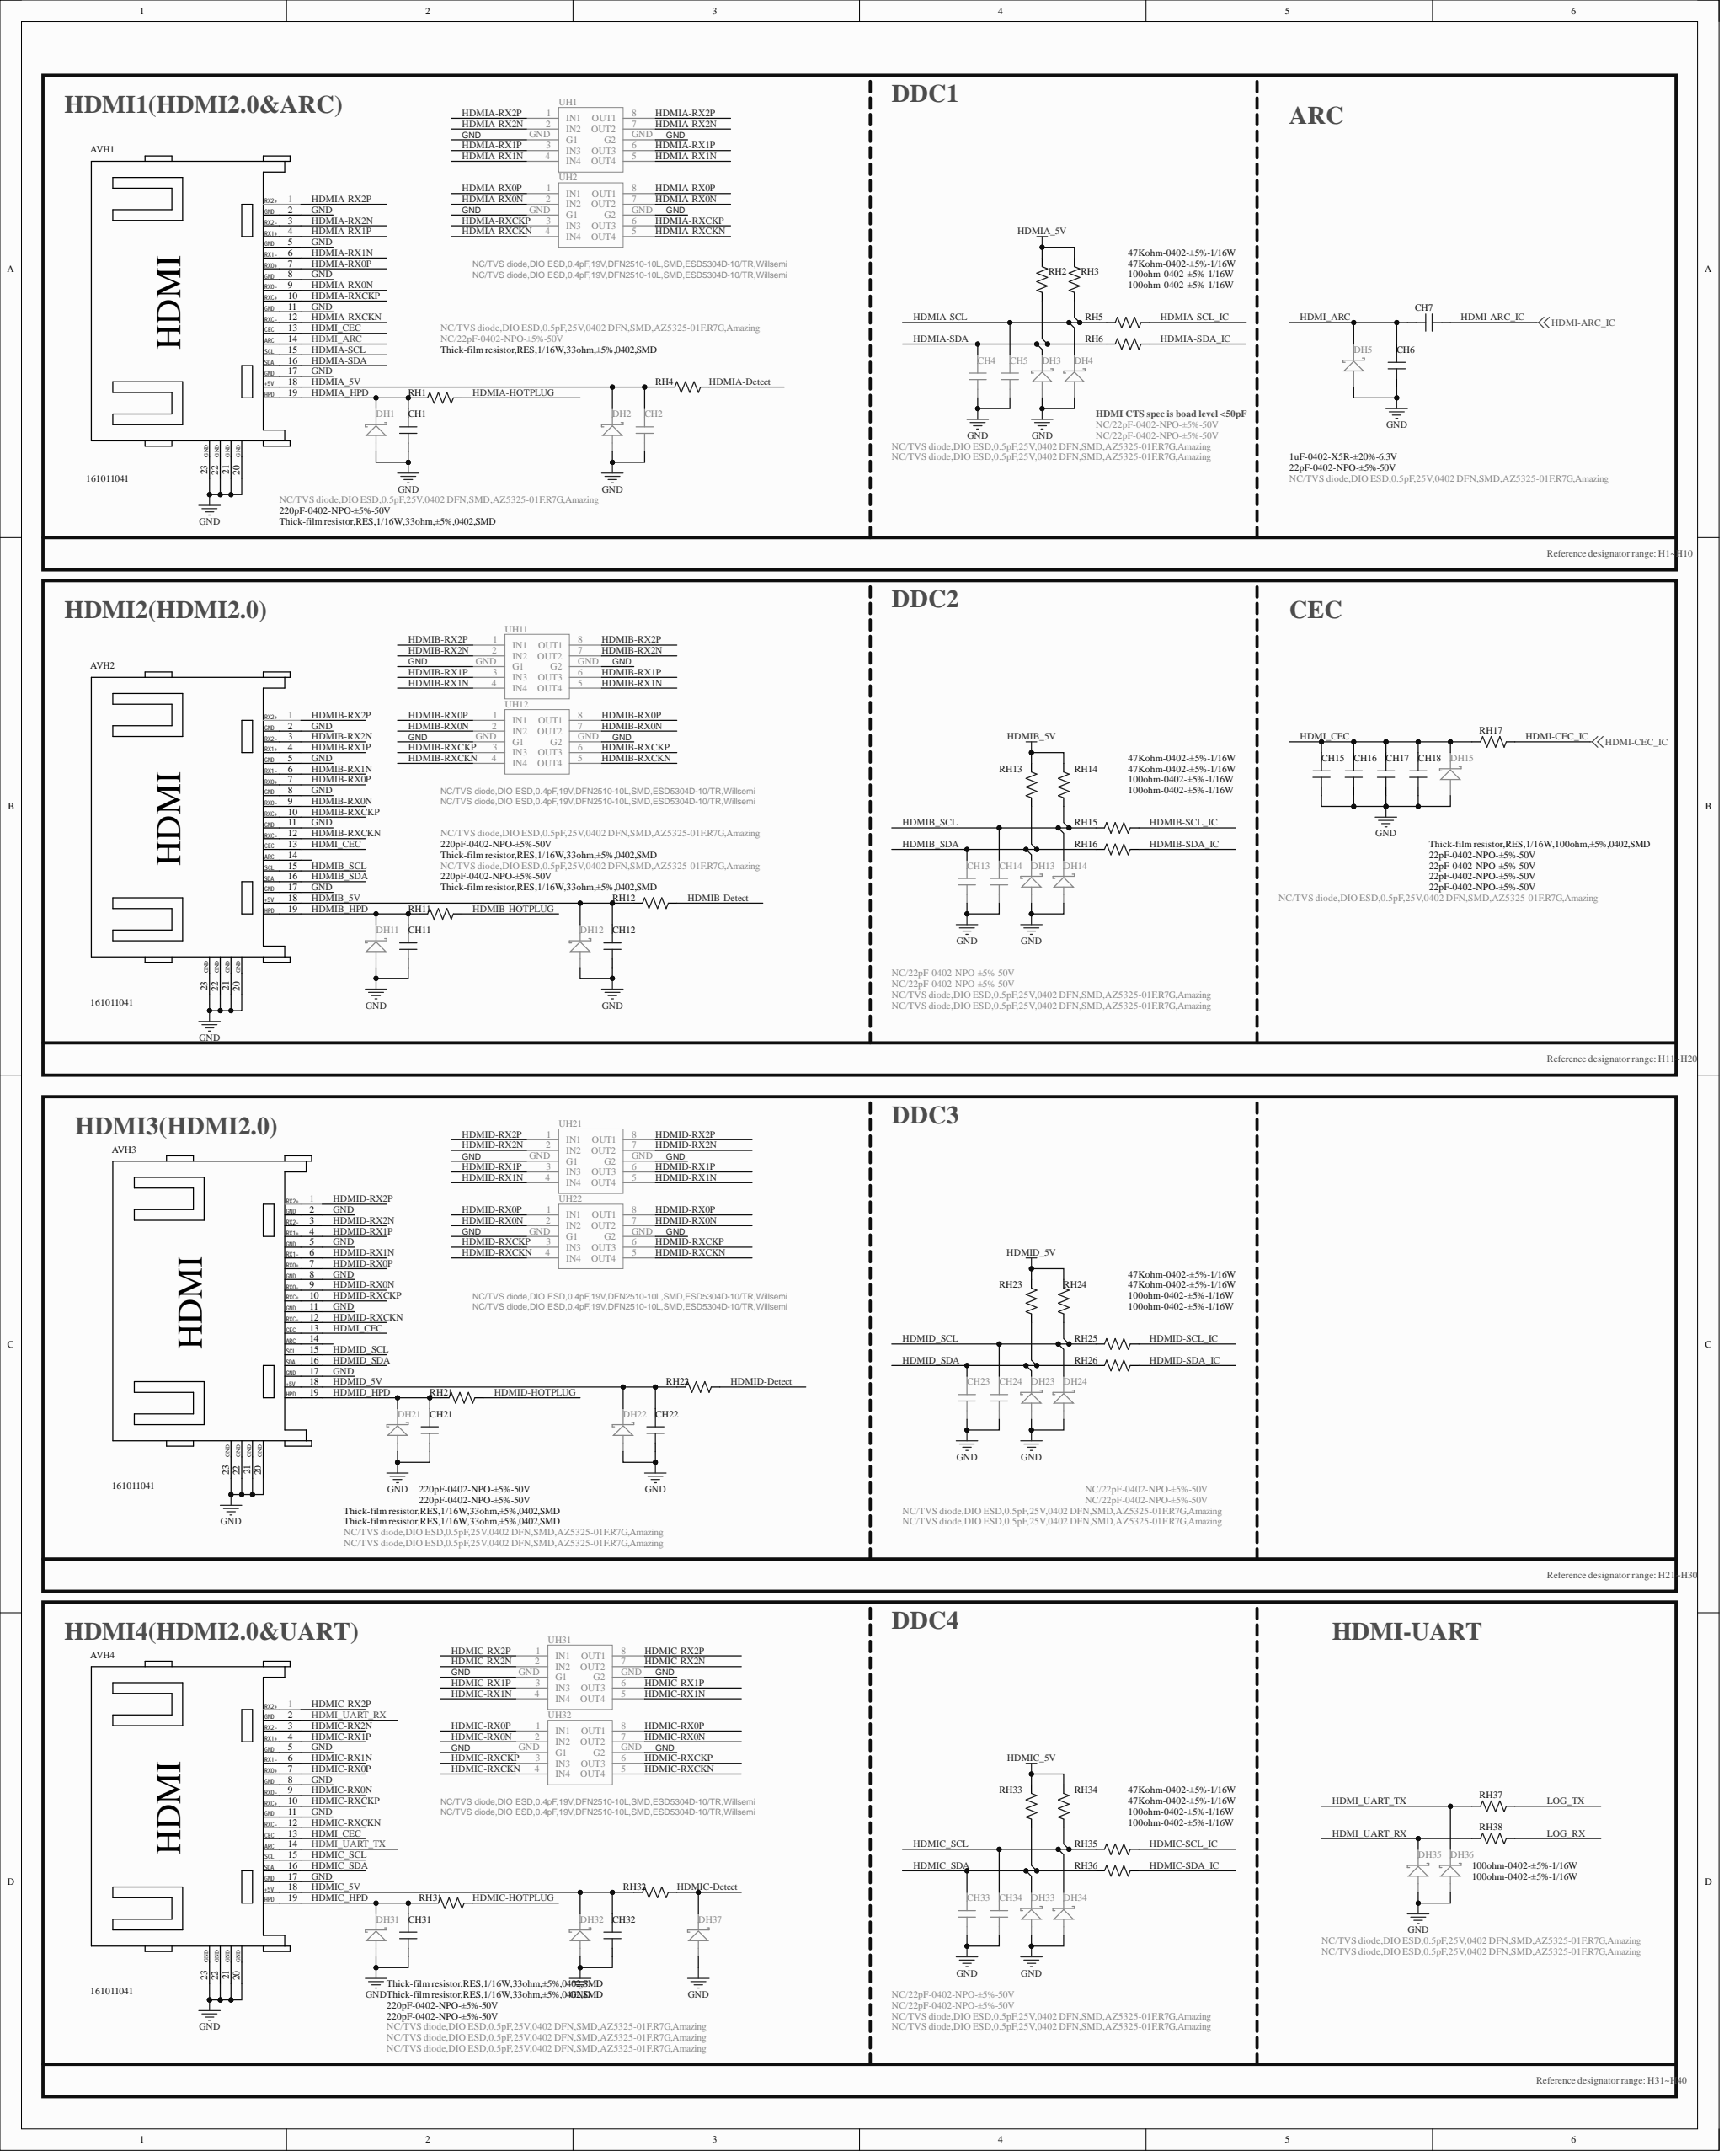Circuit board | Altium Designer | 1029 parts | 642 nets | one sheet of the schematic
Parts on this sheet (reference | value | footprint):
AVH1 | 161011041 | HDMI-HS-1
AVH2 | 161011041 | HDMI-HS-1
AVH3 | 161011041 | HDMI-HS-1
AVH4 | 161011041 | HDMI-HS-1
CH1 | 220pF-0402-NPO-±5%-50V | C0402
CH2 | NC/22pF-0402-NPO-±5%-50V | C0402
CH4 | NC/22pF-0402-NPO-±5%-50V | C0402
CH5 | NC/22pF-0402-NPO-±5%-50V | C0402
CH6 | 22pF-0402-NPO-±5%-50V | C0402
CH7 | 1uF-0402-X5R-±20%-6.3V | C0402
CH11 | 220pF-0402-NPO-±5%-50V | C0402
CH12 | 220pF-0402-NPO-±5%-50V | C0402
CH13 | NC/22pF-0402-NPO-±5%-50V | C0402
CH14 | NC/22pF-0402-NPO-±5%-50V | C0402
CH15 | 22pF-0402-NPO-±5%-50V | C0402
CH16 | 22pF-0402-NPO-±5%-50V | C0402
CH17 | 22pF-0402-NPO-±5%-50V | C0402
CH18 | 22pF-0402-NPO-±5%-50V | C0402
CH21 | 220pF-0402-NPO-±5%-50V | C0402
CH22 | 220pF-0402-NPO-±5%-50V | C0402
CH23 | NC/22pF-0402-NPO-±5%-50V | C0402
CH24 | NC/22pF-0402-NPO-±5%-50V | C0402
CH31 | 220pF-0402-NPO-±5%-50V | C0402
CH32 | 220pF-0402-NPO-±5%-50V | C0402
CH33 | NC/22pF-0402-NPO-±5%-50V | C0402
CH34 | NC/22pF-0402-NPO-±5%-50V | C0402
DH1 | NC/TVS diode,DIO ESD,0.5pF,25V,0402 DFN,SMD,AZ5325-01F.R7G,Amazing | DIODE-S0402
DH2 | NC/TVS diode,DIO ESD,0.5pF,25V,0402 DFN,SMD,AZ5325-01F.R7G,Amazing | DIODE-S0402
DH3 | NC/TVS diode,DIO ESD,0.5pF,25V,0402 DFN,SMD,AZ5325-01F.R7G,Amazing | DIODE-S0402
DH4 | NC/TVS diode,DIO ESD,0.5pF,25V,0402 DFN,SMD,AZ5325-01F.R7G,Amazing | DIODE-S0402
DH5 | NC/TVS diode,DIO ESD,0.5pF,25V,0402 DFN,SMD,AZ5325-01F.R7G,Amazing | DIODE-S0402
DH11 | NC/TVS diode,DIO ESD,0.5pF,25V,0402 DFN,SMD,AZ5325-01F.R7G,Amazing | DIODE-S0402
DH12 | NC/TVS diode,DIO ESD,0.5pF,25V,0402 DFN,SMD,AZ5325-01F.R7G,Amazing | DIODE-S0402
DH13 | NC/TVS diode,DIO ESD,0.5pF,25V,0402 DFN,SMD,AZ5325-01F.R7G,Amazing | DIODE-S0402
DH14 | NC/TVS diode,DIO ESD,0.5pF,25V,0402 DFN,SMD,AZ5325-01F.R7G,Amazing | DIODE-S0402
DH15 | NC/TVS diode,DIO ESD,0.5pF,25V,0402 DFN,SMD,AZ5325-01F.R7G,Amazing | DIODE-S0402
DH21 | NC/TVS diode,DIO ESD,0.5pF,25V,0402 DFN,SMD,AZ5325-01F.R7G,Amazing | DIODE-S0402
DH22 | NC/TVS diode,DIO ESD,0.5pF,25V,0402 DFN,SMD,AZ5325-01F.R7G,Amazing | DIODE-S0402
DH23 | NC/TVS diode,DIO ESD,0.5pF,25V,0402 DFN,SMD,AZ5325-01F.R7G,Amazing | DIODE-S0402
DH24 | NC/TVS diode,DIO ESD,0.5pF,25V,0402 DFN,SMD,AZ5325-01F.R7G,Amazing | DIODE-S0402
DH31 | NC/TVS diode,DIO ESD,0.5pF,25V,0402 DFN,SMD,AZ5325-01F.R7G,Amazing | DIODE-S0402
DH32 | NC/TVS diode,DIO ESD,0.5pF,25V,0402 DFN,SMD,AZ5325-01F.R7G,Amazing | DIODE-S0402
DH33 | NC/TVS diode,DIO ESD,0.5pF,25V,0402 DFN,SMD,AZ5325-01F.R7G,Amazing | DIODE-S0402
DH34 | NC/TVS diode,DIO ESD,0.5pF,25V,0402 DFN,SMD,AZ5325-01F.R7G,Amazing | DIODE-S0402
DH35 | NC/TVS diode,DIO ESD,0.5pF,25V,0402 DFN,SMD,AZ5325-01F.R7G,Amazing | DIODE-S0402
DH36 | NC/TVS diode,DIO ESD,0.5pF,25V,0402 DFN,SMD,AZ5325-01F.R7G,Amazing | DIODE-S0402
DH37 | NC/TVS diode,DIO ESD,0.5pF,25V,0402 DFN,SMD,AZ5325-01F.R7G,Amazing | DIODE-S0402
RH1 | Thick-film resistor,RES,1/16W,33ohm,±5%,0402,SMD | R0402
RH2 | 47Kohm-0402-±5%-1/16W | R0402
RH3 | 47Kohm-0402-±5%-1/16W | R0402
RH4 | Thick-film resistor,RES,1/16W,33ohm,±5%,0402,SMD | R0402
RH5 | 100ohm-0402-±5%-1/16W | R0402
RH6 | 100ohm-0402-±5%-1/16W | R0402
RH11 | Thick-film resistor,RES,1/16W,33ohm,±5%,0402,SMD | R0402
RH12 | Thick-film resistor,RES,1/16W,33ohm,±5%,0402,SMD | R0402
RH13 | 47Kohm-0402-±5%-1/16W | R0402
RH14 | 47Kohm-0402-±5%-1/16W | R0402
RH15 | 100ohm-0402-±5%-1/16W | R0402
RH16 | 100ohm-0402-±5%-1/16W | R0402
RH17 | Thick-film resistor,RES,1/16W,100ohm,±5%,0402,SMD | R0402
RH21 | Thick-film resistor,RES,1/16W,33ohm,±5%,0402,SMD | R0402
RH22 | Thick-film resistor,RES,1/16W,33ohm,±5%,0402,SMD | R0402
RH23 | 47Kohm-0402-±5%-1/16W | R0402
RH24 | 47Kohm-0402-±5%-1/16W | R0402
RH25 | 100ohm-0402-±5%-1/16W | R0402
RH26 | 100ohm-0402-±5%-1/16W | R0402
RH31 | Thick-film resistor,RES,1/16W,33ohm,±5%,0402,SMD | R0402
RH32 | Thick-film resistor,RES,1/16W,33ohm,±5%,0402,SMD | R0402
RH33 | 47Kohm-0402-±5%-1/16W | R0402
RH34 | 47Kohm-0402-±5%-1/16W | R0402
RH35 | 100ohm-0402-±5%-1/16W | R0402
RH36 | 100ohm-0402-±5%-1/16W | R0402
RH37 | 100ohm-0402-±5%-1/16W | R0402
RH38 | 100ohm-0402-±5%-1/16W | R0402
UH1 | NC/TVS diode,DIO ESD,0.4pF,19V,DFN2510-10L,SMD,ESD5304D-10/TR,Willsemi | RCL0524P
UH2 | NC/TVS diode,DIO ESD,0.4pF,19V,DFN2510-10L,SMD,ESD5304D-10/TR,Willsemi | RCL0524P
UH11 | NC/TVS diode,DIO ESD,0.4pF,19V,DFN2510-10L,SMD,ESD5304D-10/TR,Willsemi | RCL0524P
UH12 | NC/TVS diode,DIO ESD,0.4pF,19V,DFN2510-10L,SMD,ESD5304D-10/TR,Willsemi | RCL0524P
UH21 | NC/TVS diode,DIO ESD,0.4pF,19V,DFN2510-10L,SMD,ESD5304D-10/TR,Willsemi | RCL0524P
UH22 | NC/TVS diode,DIO ESD,0.4pF,19V,DFN2510-10L,SMD,ESD5304D-10/TR,Willsemi | RCL0524P
UH31 | NC/TVS diode,DIO ESD,0.4pF,19V,DFN2510-10L,SMD,ESD5304D-10/TR,Willsemi | RCL0524P
UH32 | NC/TVS diode,DIO ESD,0.4pF,19V,DFN2510-10L,SMD,ESD5304D-10/TR,Willsemi | RCL0524P
Nets of these parts (net: part-pin ...):
LOG_TX: RH37-2
LOG_RX: RH38-2
HDMID_SDA: CH23-1 DH23-K RH23-1 RH26-1 AVH3-16
HDMID_SCL: CH24-1 DH24-K RH24-1 RH25-1 AVH3-15
HDMID_HPD: CH21-1 DH21-K RH21-2 AVH3-19
HDMID_5V: CH22-1 DH22-K RH22-2 RH23-2 RH24-2 AVH3-18
HDMID-SDA_IC: RH26-2
HDMID-SCL_IC: RH25-2
HDMID-RXCKP: UH22-3 UH22-6 AVH3-10
HDMID-RXCKN: UH22-4 UH22-5 AVH3-12
HDMID-RX2P: UH21-1 UH21-8 AVH3-1
HDMID-RX2N: UH21-2 UH21-7 AVH3-3
HDMID-RX1P: UH21-3 UH21-6 AVH3-4
HDMID-RX1N: UH21-4 UH21-5 AVH3-6
HDMID-RX0P: UH22-1 UH22-8 AVH3-7
HDMID-RX0N: UH22-2 UH22-7 AVH3-9
HDMID-HOTPLUG: RH21-1
HDMID-Detect: RH22-1
HDMIC_SDA: CH33-1 DH33-K RH33-1 RH36-1 AVH4-16
HDMIC_SCL: CH34-1 DH34-K RH34-1 RH35-1 AVH4-15
HDMIC_HPD: CH31-1 DH31-K RH31-2 AVH4-19
HDMIC_5V: CH32-1 DH32-K RH32-2 RH33-2 RH34-2 AVH4-18
HDMIC-SDA_IC: RH36-2
HDMIC-SCL_IC: RH35-2
HDMIC-RXCKP: UH32-3 UH32-6 AVH4-10
HDMIC-RXCKN: UH32-4 UH32-5 AVH4-12
HDMIC-RX2P: UH31-1 UH31-8 AVH4-1
HDMIC-RX2N: UH31-2 UH31-7 AVH4-3
HDMIC-RX1P: UH31-3 UH31-6 AVH4-4
HDMIC-RX1N: UH31-4 UH31-5 AVH4-6
HDMIC-RX0P: UH32-1 UH32-8 AVH4-7
HDMIC-RX0N: UH32-2 UH32-7 AVH4-9
HDMIC-HOTPLUG: RH31-1
HDMIC-Detect: DH37-K RH32-1
HDMIB_SDA: CH13-1 DH13-K RH13-1 RH16-1 AVH2-16
HDMIB_SCL: CH14-1 DH14-K RH14-1 RH15-1 AVH2-15
HDMIB_HPD: CH11-1 DH11-K RH11-2 AVH2-19
HDMIB_5V: CH12-1 DH12-K RH12-2 RH13-2 RH14-2 AVH2-18
HDMIB-SDA_IC: RH16-2
HDMIB-SCL_IC: RH15-2
HDMIB-RXCKP: UH12-3 UH12-6 AVH2-10
HDMIB-RXCKN: UH12-4 UH12-5 AVH2-12
HDMIB-RX2P: UH11-1 UH11-8 AVH2-1
HDMIB-RX2N: UH11-2 UH11-7 AVH2-3
HDMIB-RX1P: UH11-3 UH11-6 AVH2-4
HDMIB-RX1N: UH11-4 UH11-5 AVH2-6
HDMIB-RX0P: UH12-1 UH12-8 AVH2-7
HDMIB-RX0N: UH12-2 UH12-7 AVH2-9
HDMIB-HOTPLUG: RH11-1
HDMIB-Detect: RH12-1
HDMIA_HPD: CH1-1 DH1-K RH1-2 AVH1-19
HDMIA_5V: CH2-1 DH2-K RH2-2 RH3-2 RH4-2 AVH1-18
HDMIA-SDA_IC: RH6-2
HDMIA-SDA: CH4-1 DH3-K RH2-1 RH6-1 AVH1-16
HDMIA-SCL_IC: RH5-2
HDMIA-SCL: CH5-1 DH4-K RH3-1 RH5-1 AVH1-15
HDMIA-RXCKP: UH2-3 UH2-6 AVH1-10
HDMIA-RXCKN: UH2-4 UH2-5 AVH1-12
HDMIA-RX2P: UH1-1 UH1-8 AVH1-1
HDMIA-RX2N: UH1-2 UH1-7 AVH1-3
HDMIA-RX1P: UH1-3 UH1-6 AVH1-4
HDMIA-RX1N: UH1-4 UH1-5 AVH1-6
HDMIA-RX0P: UH2-1 UH2-8 AVH1-7
HDMIA-RX0N: UH2-2 UH2-7 AVH1-9
HDMIA-HOTPLUG: RH1-1
HDMIA-Detect: RH4-1
HDMI_UART_TX: DH36-K RH37-1 AVH4-14
HDMI_UART_RX: DH35-K RH38-1 AVH4-2
HDMI_CEC: CH15-2 CH16-2 CH17-2 CH18-2 DH15-K RH17-1 AVH1-13 AVH2-13 AVH3-13 AVH4-13
HDMI_ARC: CH6-1 CH7-1 DH5-K AVH1-14
HDMI-CEC_IC: RH17-2
HDMI-ARC_IC: CH7-2
GND: CH1-2 CH2-2 CH4-2 CH5-2 CH6-2 CH11-2 CH12-2 CH13-2 CH14-2 CH15-1 CH16-1 CH17-1 CH18-1 CH21-2 CH22-2 CH23-2 CH24-2 CH31-2 CH32-2 CH33-2 CH34-2 DH1-A DH2-A DH3-A DH4-A DH5-A DH11-A DH12-A DH13-A DH14-A DH15-A DH21-A DH22-A DH23-A DH24-A DH31-A DH32-A DH33-A DH34-A DH35-A DH36-A DH37-A UH1-GND UH2-GND UH11-GND UH12-GND UH21-GND UH22-GND UH31-GND UH32-GND AVH1-2 AVH1-5 AVH1-8 AVH1-11 AVH1-17 AVH1-20 AVH1-21 AVH1-22 AVH1-23 AVH2-2 AVH2-5 AVH2-8 AVH2-11 AVH2-17 AVH2-20 AVH2-21 AVH2-22 AVH2-23 AVH3-2 AVH3-5 AVH3-8 AVH3-11 AVH3-17 AVH3-20 AVH3-21 AVH3-22 AVH3-23 AVH4-5 AVH4-8 AVH4-11 AVH4-17 AVH4-20 AVH4-21 AVH4-22 AVH4-23